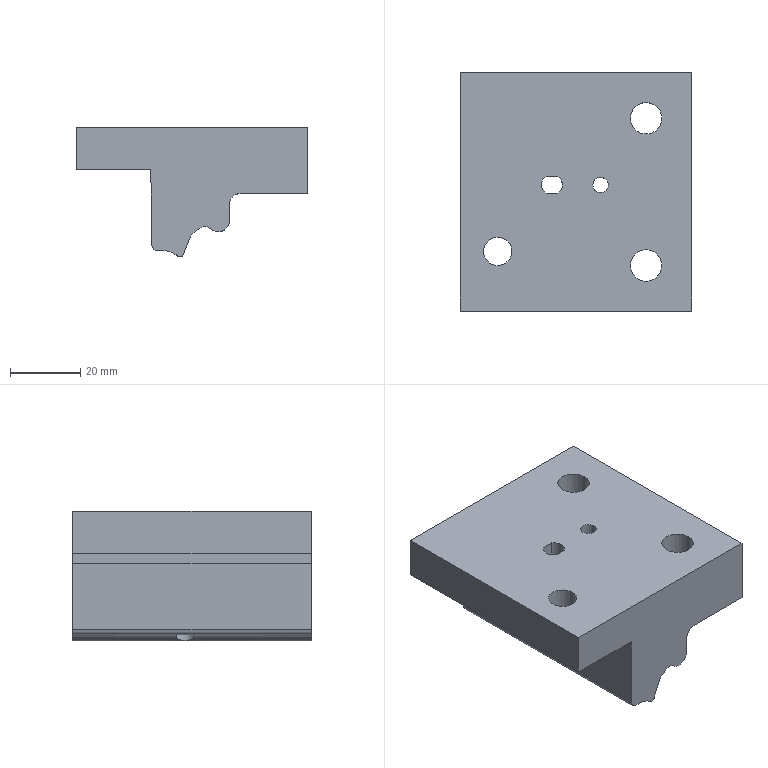Part | 1 solid | 47 faces | box 66.004 x 68 x 37.027 mm | volume 88999 mm3 | cylinder 25 | plane 22 | commonest cylinder face diameters 6 x4 9 x4 14 x4 4.415 x2 6.401 x2 8.1 x2